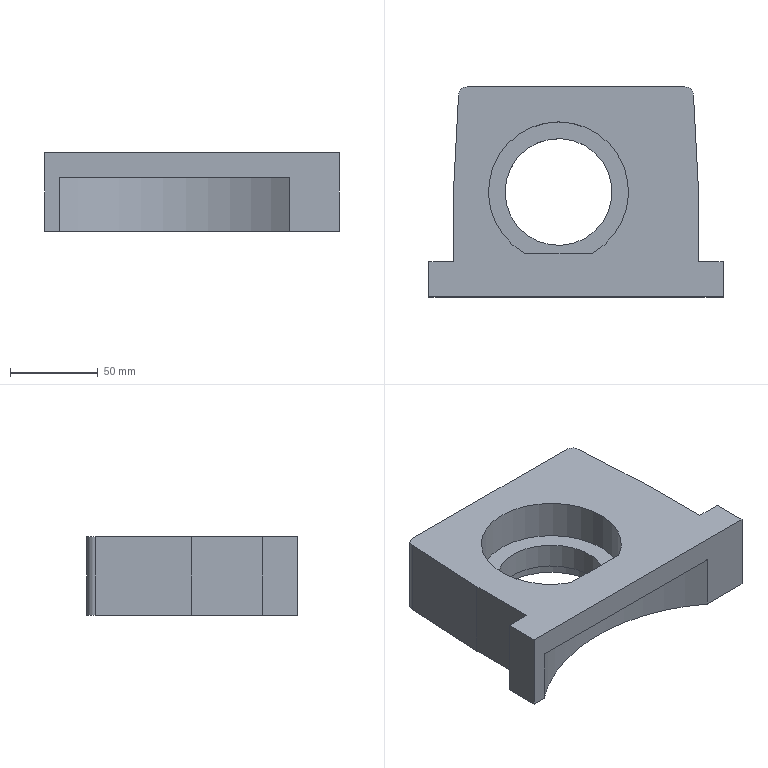Part | STEP file | SLIDE2-3_id590_x_t | 1 solid | 22 faces | box 168 x 120 x 45 mm | volume 525996 mm3 | plane 16 | cylinder 6 | commonest cylinder face diameters 10 x2 61 x1 71 x1 80 x1 217 x1
STEP:
#1=CARTESIAN_POINT('',(-60.5,0.,123.003));
#2=VERTEX_POINT('',#1);
#3=CARTESIAN_POINT('',(-30.,0.,123.003));
#4=DIRECTION('',(0.,0.,1.));
#5=DIRECTION('',(-1.,0.,0.));
#6=AXIS2_PLACEMENT_3D('',#3,#4,#5);
#7=CIRCLE('',#6,30.5);
#8=EDGE_CURVE('',#2,#2,#7,.T.);
#9=ORIENTED_EDGE('',*,*,#8,.T.);
#10=EDGE_LOOP('',(#9));
#11=FACE_BOUND('',#10,.T.);
#12=CARTESIAN_POINT('',(-65.5,0.,123.003));
#13=VERTEX_POINT('',#12);
#14=CARTESIAN_POINT('',(-30.,0.,123.003));
#15=DIRECTION('',(0.,0.,-1.));
#16=DIRECTION('',(-1.,0.,0.));
#17=AXIS2_PLACEMENT_3D('',#14,#15,#16);
#18=CIRCLE('',#17,35.5);
#19=EDGE_CURVE('',#13,#13,#18,.T.);
#20=ORIENTED_EDGE('',*,*,#19,.T.);
#21=EDGE_LOOP('',(#20));
#22=FACE_BOUND('',#21,.T.);
#23=CARTESIAN_POINT('',(50.,60.,123.003));
#24=DIRECTION('',(0.,0.,-1.));
#25=DIRECTION('',(-1.,0.,0.));
#26=AXIS2_PLACEMENT_3D('',#23,#24,#25);
#27=PLANE('',#26);
#28=ADVANCED_FACE('',(#11,#22),#27,.T.);
#29=ORIENTED_EDGE('',*,*,#19,.F.);
#30=EDGE_LOOP('',(#29));
#31=FACE_BOUND('',#30,.T.);
#32=CARTESIAN_POINT('',(-65.5,0.,115.003));
#33=VERTEX_POINT('',#32);
#34=CARTESIAN_POINT('',(-30.,0.,115.003));
#35=DIRECTION('',(0.,0.,-1.));
#36=DIRECTION('',(-1.,0.,0.));
#37=AXIS2_PLACEMENT_3D('',#34,#35,#36);
#38=CIRCLE('',#37,35.5);
#39=EDGE_CURVE('',#33,#33,#38,.T.);
#40=ORIENTED_EDGE('',*,*,#39,.T.);
#41=EDGE_LOOP('',(#40));
#42=FACE_BOUND('',#41,.T.);
#43=CARTESIAN_POINT('',(-30.,0.,115.003));
#44=DIRECTION('',(0.,0.,-1.));
#45=DIRECTION('',(-1.,0.,0.));
#46=AXIS2_PLACEMENT_3D('',#43,#44,#45);
#47=CYLINDRICAL_SURFACE('',#46,35.5);
#48=ADVANCED_FACE('',(#31,#42),#47,.F.);
#49=ORIENTED_EDGE('',*,*,#8,.F.);
#50=EDGE_LOOP('',(#49));
#51=FACE_BOUND('',#50,.T.);
#52=CARTESIAN_POINT('',(-60.5,0.,137.503));
#53=VERTEX_POINT('',#52);
#54=CARTESIAN_POINT('',(-30.,0.,137.503));
#55=DIRECTION('',(0.,0.,1.));
#56=DIRECTION('',(-1.,0.,0.));
#57=AXIS2_PLACEMENT_3D('',#54,#55,#56);
#58=CIRCLE('',#57,30.5);
#59=EDGE_CURVE('',#53,#53,#58,.T.);
#60=ORIENTED_EDGE('',*,*,#59,.T.);
#61=EDGE_LOOP('',(#60));
#62=FACE_BOUND('',#61,.T.);
#63=CARTESIAN_POINT('',(-30.,0.,123.003));
#64=DIRECTION('',(0.,0.,-1.));
#65=DIRECTION('',(-1.,0.,0.));
#66=AXIS2_PLACEMENT_3D('',#63,#64,#65);
#67=CYLINDRICAL_SURFACE('',#66,30.5);
#68=ADVANCED_FACE('',(#51,#62),#67,.F.);
#69=CARTESIAN_POINT('',(35.892,-60.,146.));
#70=VERTEX_POINT('',#69);
#71=CARTESIAN_POINT('',(-95.892,-60.,146.));
#72=VERTEX_POINT('',#71);
#73=CARTESIAN_POINT('',(-30.,-146.2,146.));
#74=DIRECTION('',(0.,0.,1.));
#75=DIRECTION('',(1.,0.,0.));
#76=AXIS2_PLACEMENT_3D('',#73,#74,#75);
#77=CIRCLE('',#76,108.5);
#78=EDGE_CURVE('',#70,#72,#77,.T.);
#79=ORIENTED_EDGE('',*,*,#78,.T.);
#80=CARTESIAN_POINT('',(-95.892,-60.,115.003));
#81=VERTEX_POINT('',#80);
#82=CARTESIAN_POINT('',(-95.892,-60.,115.003));
#83=DIRECTION('',(0.,0.,1.));
#84=VECTOR('',#83,1.);
#85=LINE('',#82,#84);
#86=EDGE_CURVE('',#81,#72,#85,.T.);
#87=ORIENTED_EDGE('',*,*,#86,.F.);
#88=CARTESIAN_POINT('',(35.892,-60.,115.003));
#89=VERTEX_POINT('',#88);
#90=CARTESIAN_POINT('',(-30.,-146.2,115.003));
#91=DIRECTION('',(0.,0.,-1.));
#92=DIRECTION('',(1.,0.,0.));
#93=AXIS2_PLACEMENT_3D('',#90,#91,#92);
#94=CIRCLE('',#93,108.5);
#95=EDGE_CURVE('',#81,#89,#94,.T.);
#96=ORIENTED_EDGE('',*,*,#95,.T.);
#97=CARTESIAN_POINT('',(35.892,-60.,115.003));
#98=DIRECTION('',(0.,0.,-1.));
#99=VECTOR('',#98,1.);
#100=LINE('',#97,#99);
#101=EDGE_CURVE('',#70,#89,#100,.T.);
#102=ORIENTED_EDGE('',*,*,#101,.F.);
#103=EDGE_LOOP('',(#79,#87,#96,#102));
#104=FACE_OUTER_BOUND('',#103,.T.);
#105=CARTESIAN_POINT('',(-30.,-146.2,146.));
#106=DIRECTION('',(0.,0.,1.));
#107=DIRECTION('',(1.,0.,0.));
#108=AXIS2_PLACEMENT_3D('',#105,#106,#107);
#109=CYLINDRICAL_SURFACE('',#108,108.5);
#110=ADVANCED_FACE('',(#104),#109,.F.);
#111=CARTESIAN_POINT('',(-98.,-60.,146.));
#112=DIRECTION('',(1.,0.,0.));
#113=VECTOR('',#112,1.);
#114=LINE('',#111,#113);
#115=EDGE_CURVE('',#72,#70,#114,.T.);
#116=ORIENTED_EDGE('',*,*,#115,.F.);
#117=ORIENTED_EDGE('',*,*,#78,.F.);
#118=EDGE_LOOP('',(#116,#117));
#119=FACE_OUTER_BOUND('',#118,.T.);
#120=CARTESIAN_POINT('',(0.,-40.,146.));
#121=DIRECTION('',(0.,0.,1.));
#122=DIRECTION('',(1.,0.,0.));
#123=AXIS2_PLACEMENT_3D('',#120,#121,#122);
#124=PLANE('',#123);
#125=ADVANCED_FACE('',(#119),#124,.F.);
#126=ORIENTED_EDGE('',*,*,#39,.F.);
#127=EDGE_LOOP('',(#126));
#128=FACE_BOUND('',#127,.T.);
#129=CARTESIAN_POINT('',(50.,-40.,115.003));
#130=VERTEX_POINT('',#129);
#131=CARTESIAN_POINT('',(50.,0.05468,115.003));
#132=VERTEX_POINT('',#131);
#133=CARTESIAN_POINT('',(50.,-50.,115.003));
#134=DIRECTION('',(0.,1.,0.));
#135=VECTOR('',#134,1.);
#136=LINE('',#133,#135);
#137=EDGE_CURVE('',#130,#132,#136,.T.);
#138=ORIENTED_EDGE('',*,*,#137,.F.);
#139=CARTESIAN_POINT('',(64.,-40.,115.003));
#140=VERTEX_POINT('',#139);
#141=CARTESIAN_POINT('',(58.,-40.,115.003));
#142=DIRECTION('',(-1.,0.,0.));
#143=VECTOR('',#142,1.);
#144=LINE('',#141,#143);
#145=EDGE_CURVE('',#140,#130,#144,.T.);
#146=ORIENTED_EDGE('',*,*,#145,.F.);
#147=CARTESIAN_POINT('',(64.,-60.,115.003));
#148=VERTEX_POINT('',#147);
#149=CARTESIAN_POINT('',(64.,-60.,115.003));
#150=DIRECTION('',(0.,1.,0.));
#151=VECTOR('',#150,1.);
#152=LINE('',#149,#151);
#153=EDGE_CURVE('',#148,#140,#152,.T.);
#154=ORIENTED_EDGE('',*,*,#153,.F.);
#155=CARTESIAN_POINT('',(-98.,-60.,115.003));
#156=DIRECTION('',(1.,0.,0.));
#157=VECTOR('',#156,1.);
#158=LINE('',#155,#157);
#159=EDGE_CURVE('',#89,#148,#158,.T.);
#160=ORIENTED_EDGE('',*,*,#159,.F.);
#161=ORIENTED_EDGE('',*,*,#95,.F.);
#162=CARTESIAN_POINT('',(-104.,-60.,115.003));
#163=VERTEX_POINT('',#162);
#164=CARTESIAN_POINT('',(-98.,-60.,115.003));
#165=DIRECTION('',(1.,0.,0.));
#166=VECTOR('',#165,1.);
#167=LINE('',#164,#166);
#168=EDGE_CURVE('',#163,#81,#167,.T.);
#169=ORIENTED_EDGE('',*,*,#168,.F.);
#170=CARTESIAN_POINT('',(-104.,-40.,115.003));
#171=VERTEX_POINT('',#170);
#172=CARTESIAN_POINT('',(-104.,-50.,115.003));
#173=DIRECTION('',(0.,-1.,0.));
#174=VECTOR('',#173,1.);
#175=LINE('',#172,#174);
#176=EDGE_CURVE('',#171,#163,#175,.T.);
#177=ORIENTED_EDGE('',*,*,#176,.F.);
#178=CARTESIAN_POINT('',(-90.,-40.,115.003));
#179=VERTEX_POINT('',#178);
#180=CARTESIAN_POINT('',(-90.,-40.,115.003));
#181=DIRECTION('',(-1.,0.,0.));
#182=VECTOR('',#181,1.);
#183=LINE('',#180,#182);
#184=EDGE_CURVE('',#179,#171,#183,.T.);
#185=ORIENTED_EDGE('',*,*,#184,.F.);
#186=CARTESIAN_POINT('',(-90.,0.05468,115.003));
#187=VERTEX_POINT('',#186);
#188=CARTESIAN_POINT('',(-90.,60.,115.003));
#189=DIRECTION('',(0.,-1.,0.));
#190=VECTOR('',#189,1.);
#191=LINE('',#188,#190);
#192=EDGE_CURVE('',#187,#179,#191,.T.);
#193=ORIENTED_EDGE('',*,*,#192,.F.);
#194=CARTESIAN_POINT('',(-87.107,55.262,115.003));
#195=VERTEX_POINT('',#194);
#196=CARTESIAN_POINT('',(-87.107,55.262,115.003));
#197=DIRECTION('',(0.05234,0.9986,0.));
#198=VECTOR('',#197,1.);
#199=LINE('',#196,#198);
#200=EDGE_CURVE('',#187,#195,#199,.T.);
#201=ORIENTED_EDGE('',*,*,#200,.T.);
#202=CARTESIAN_POINT('',(-82.114,60.,115.003));
#203=VERTEX_POINT('',#202);
#204=CARTESIAN_POINT('',(-82.114,55.,115.003));
#205=DIRECTION('',(0.,0.,1.));
#206=DIRECTION('',(-1.,0.,0.));
#207=AXIS2_PLACEMENT_3D('',#204,#205,#206);
#208=CIRCLE('',#207,5.);
#209=EDGE_CURVE('',#203,#195,#208,.T.);
#210=ORIENTED_EDGE('',*,*,#209,.F.);
#211=CARTESIAN_POINT('',(42.114,60.,115.003));
#212=VERTEX_POINT('',#211);
#213=CARTESIAN_POINT('',(50.,60.,115.003));
#214=DIRECTION('',(-1.,0.,0.));
#215=VECTOR('',#214,1.);
#216=LINE('',#213,#215);
#217=EDGE_CURVE('',#212,#203,#216,.T.);
#218=ORIENTED_EDGE('',*,*,#217,.F.);
#219=CARTESIAN_POINT('',(47.107,55.262,115.003));
#220=VERTEX_POINT('',#219);
#221=CARTESIAN_POINT('',(42.114,55.,115.003));
#222=DIRECTION('',(0.,0.,1.));
#223=DIRECTION('',(-1.,0.,0.));
#224=AXIS2_PLACEMENT_3D('',#221,#222,#223);
#225=CIRCLE('',#224,5.);
#226=EDGE_CURVE('',#220,#212,#225,.T.);
#227=ORIENTED_EDGE('',*,*,#226,.F.);
#228=CARTESIAN_POINT('',(50.,0.05468,115.003));
#229=DIRECTION('',(0.05234,-0.9986,0.));
#230=VECTOR('',#229,1.);
#231=LINE('',#228,#230);
#232=EDGE_CURVE('',#220,#132,#231,.T.);
#233=ORIENTED_EDGE('',*,*,#232,.T.);
#234=EDGE_LOOP('',(#138,#146,#154,#160,#161,#169,#177,#185,#193,#201,#210,#218,#227,#233));
#235=FACE_BOUND('',#234,.T.);
#236=CARTESIAN_POINT('',(50.5,0.,115.003));
#237=DIRECTION('',(0.,0.,1.));
#238=DIRECTION('',(1.,0.,0.));
#239=AXIS2_PLACEMENT_3D('',#236,#237,#238);
#240=PLANE('',#239);
#241=ADVANCED_FACE('',(#128,#235),#240,.F.);
#242=ORIENTED_EDGE('',*,*,#59,.F.);
#243=EDGE_LOOP('',(#242));
#244=FACE_BOUND('',#243,.T.);
#245=CARTESIAN_POINT('',(-10.635,-35.,137.503));
#246=VERTEX_POINT('',#245);
#247=CARTESIAN_POINT('',(-49.365,-35.,137.503));
#248=VERTEX_POINT('',#247);
#249=CARTESIAN_POINT('',(-30.,0.,137.503));
#250=DIRECTION('',(0.,0.,1.));
#251=DIRECTION('',(-1.,0.,0.));
#252=AXIS2_PLACEMENT_3D('',#249,#250,#251);
#253=CIRCLE('',#252,40.);
#254=EDGE_CURVE('',#246,#248,#253,.T.);
#255=ORIENTED_EDGE('',*,*,#254,.T.);
#256=CARTESIAN_POINT('',(-10.635,-35.,137.503));
#257=DIRECTION('',(-1.,0.,0.));
#258=VECTOR('',#257,1.);
#259=LINE('',#256,#258);
#260=EDGE_CURVE('',#246,#248,#259,.T.);
#261=ORIENTED_EDGE('',*,*,#260,.F.);
#262=EDGE_LOOP('',(#255,#261));
#263=FACE_BOUND('',#262,.T.);
#264=CARTESIAN_POINT('',(50.,60.,137.503));
#265=DIRECTION('',(0.,0.,-1.));
#266=DIRECTION('',(-1.,0.,0.));
#267=AXIS2_PLACEMENT_3D('',#264,#265,#266);
#268=PLANE('',#267);
#269=ADVANCED_FACE('',(#244,#263),#268,.F.);
#270=CARTESIAN_POINT('',(42.114,60.,160.003));
#271=VERTEX_POINT('',#270);
#272=CARTESIAN_POINT('',(-82.114,60.,160.003));
#273=VERTEX_POINT('',#272);
#274=CARTESIAN_POINT('',(50.5,60.,160.003));
#275=DIRECTION('',(-1.,0.,0.));
#276=VECTOR('',#275,1.);
#277=LINE('',#274,#276);
#278=EDGE_CURVE('',#271,#273,#277,.T.);
#279=ORIENTED_EDGE('',*,*,#278,.F.);
#280=CARTESIAN_POINT('',(42.114,60.,115.003));
#281=DIRECTION('',(0.,0.,1.));
#282=VECTOR('',#281,1.);
#283=LINE('',#280,#282);
#284=EDGE_CURVE('',#212,#271,#283,.T.);
#285=ORIENTED_EDGE('',*,*,#284,.F.);
#286=ORIENTED_EDGE('',*,*,#217,.T.);
#287=CARTESIAN_POINT('',(-82.114,60.,115.003));
#288=DIRECTION('',(0.,0.,-1.));
#289=VECTOR('',#288,1.);
#290=LINE('',#287,#289);
#291=EDGE_CURVE('',#273,#203,#290,.T.);
#292=ORIENTED_EDGE('',*,*,#291,.F.);
#293=EDGE_LOOP('',(#279,#285,#286,#292));
#294=FACE_OUTER_BOUND('',#293,.T.);
#295=CARTESIAN_POINT('',(50.,60.,115.003));
#296=DIRECTION('',(0.,1.,0.));
#297=DIRECTION('',(0.,0.,1.));
#298=AXIS2_PLACEMENT_3D('',#295,#296,#297);
#299=PLANE('',#298);
#300=ADVANCED_FACE('',(#294),#299,.T.);
#301=ORIENTED_EDGE('',*,*,#291,.T.);
#302=ORIENTED_EDGE('',*,*,#209,.T.);
#303=CARTESIAN_POINT('',(-87.107,55.262,160.003));
#304=VERTEX_POINT('',#303);
#305=CARTESIAN_POINT('',(-87.107,55.262,115.003));
#306=DIRECTION('',(0.,0.,1.));
#307=VECTOR('',#306,1.);
#308=LINE('',#305,#307);
#309=EDGE_CURVE('',#195,#304,#308,.T.);
#310=ORIENTED_EDGE('',*,*,#309,.T.);
#311=CARTESIAN_POINT('',(-82.114,55.,160.003));
#312=DIRECTION('',(0.,0.,1.));
#313=DIRECTION('',(-1.,0.,0.));
#314=AXIS2_PLACEMENT_3D('',#311,#312,#313);
#315=CIRCLE('',#314,5.);
#316=EDGE_CURVE('',#273,#304,#315,.T.);
#317=ORIENTED_EDGE('',*,*,#316,.F.);
#318=EDGE_LOOP('',(#301,#302,#310,#317));
#319=FACE_OUTER_BOUND('',#318,.T.);
#320=CARTESIAN_POINT('',(-82.114,55.,115.003));
#321=DIRECTION('',(0.,0.,-1.));
#322=DIRECTION('',(-1.,0.,0.));
#323=AXIS2_PLACEMENT_3D('',#320,#321,#322);
#324=CYLINDRICAL_SURFACE('',#323,5.);
#325=ADVANCED_FACE('',(#319),#324,.T.);
#326=CARTESIAN_POINT('',(-90.,0.05468,160.003));
#327=VERTEX_POINT('',#326);
#328=CARTESIAN_POINT('',(-87.107,55.262,160.003));
#329=DIRECTION('',(-0.05234,-0.9986,0.));
#330=VECTOR('',#329,1.);
#331=LINE('',#328,#330);
#332=EDGE_CURVE('',#304,#327,#331,.T.);
#333=ORIENTED_EDGE('',*,*,#332,.F.);
#334=ORIENTED_EDGE('',*,*,#309,.F.);
#335=ORIENTED_EDGE('',*,*,#200,.F.);
#336=CARTESIAN_POINT('',(-90.,0.05468,115.003));
#337=DIRECTION('',(0.,0.,-1.));
#338=VECTOR('',#337,1.);
#339=LINE('',#336,#338);
#340=EDGE_CURVE('',#327,#187,#339,.T.);
#341=ORIENTED_EDGE('',*,*,#340,.F.);
#342=EDGE_LOOP('',(#333,#334,#335,#341));
#343=FACE_OUTER_BOUND('',#342,.T.);
#344=CARTESIAN_POINT('',(-87.107,55.262,115.003));
#345=DIRECTION('',(0.9986,-0.05234,0.));
#346=DIRECTION('',(0.05234,0.9986,0.));
#347=AXIS2_PLACEMENT_3D('',#344,#345,#346);
#348=PLANE('',#347);
#349=ADVANCED_FACE('',(#343),#348,.F.);
#350=CARTESIAN_POINT('',(-90.,-40.,160.003));
#351=VERTEX_POINT('',#350);
#352=CARTESIAN_POINT('',(-90.,0.,160.003));
#353=DIRECTION('',(0.,-1.,0.));
#354=VECTOR('',#353,1.);
#355=LINE('',#352,#354);
#356=EDGE_CURVE('',#327,#351,#355,.T.);
#357=ORIENTED_EDGE('',*,*,#356,.F.);
#358=ORIENTED_EDGE('',*,*,#340,.T.);
#359=ORIENTED_EDGE('',*,*,#192,.T.);
#360=CARTESIAN_POINT('',(-90.,-40.,115.003));
#361=DIRECTION('',(0.,0.,-1.));
#362=VECTOR('',#361,1.);
#363=LINE('',#360,#362);
#364=EDGE_CURVE('',#351,#179,#363,.T.);
#365=ORIENTED_EDGE('',*,*,#364,.F.);
#366=EDGE_LOOP('',(#357,#358,#359,#365));
#367=FACE_OUTER_BOUND('',#366,.T.);
#368=CARTESIAN_POINT('',(-90.,60.,115.003));
#369=DIRECTION('',(-1.,0.,0.));
#370=DIRECTION('',(0.,0.,1.));
#371=AXIS2_PLACEMENT_3D('',#368,#369,#370);
#372=PLANE('',#371);
#373=ADVANCED_FACE('',(#367),#372,.T.);
#374=ORIENTED_EDGE('',*,*,#364,.T.);
#375=ORIENTED_EDGE('',*,*,#184,.T.);
#376=CARTESIAN_POINT('',(-104.,-40.,160.003));
#377=VERTEX_POINT('',#376);
#378=CARTESIAN_POINT('',(-104.,-40.,115.003));
#379=DIRECTION('',(0.,0.,-1.));
#380=VECTOR('',#379,1.);
#381=LINE('',#378,#380);
#382=EDGE_CURVE('',#377,#171,#381,.T.);
#383=ORIENTED_EDGE('',*,*,#382,.F.);
#384=CARTESIAN_POINT('',(50.5,-40.,160.003));
#385=DIRECTION('',(-1.,0.,0.));
#386=VECTOR('',#385,1.);
#387=LINE('',#384,#386);
#388=EDGE_CURVE('',#351,#377,#387,.T.);
#389=ORIENTED_EDGE('',*,*,#388,.F.);
#390=EDGE_LOOP('',(#374,#375,#383,#389));
#391=FACE_OUTER_BOUND('',#390,.T.);
#392=CARTESIAN_POINT('',(-90.,-40.,115.003));
#393=DIRECTION('',(0.,1.,0.));
#394=DIRECTION('',(0.,0.,1.));
#395=AXIS2_PLACEMENT_3D('',#392,#393,#394);
#396=PLANE('',#395);
#397=ADVANCED_FACE('',(#391),#396,.T.);
#398=ORIENTED_EDGE('',*,*,#382,.T.);
#399=ORIENTED_EDGE('',*,*,#176,.T.);
#400=CARTESIAN_POINT('',(-104.,-60.,160.003));
#401=VERTEX_POINT('',#400);
#402=CARTESIAN_POINT('',(-104.,-60.,115.003));
#403=DIRECTION('',(0.,0.,-1.));
#404=VECTOR('',#403,1.);
#405=LINE('',#402,#404);
#406=EDGE_CURVE('',#401,#163,#405,.T.);
#407=ORIENTED_EDGE('',*,*,#406,.F.);
#408=CARTESIAN_POINT('',(-104.,0.,160.003));
#409=DIRECTION('',(0.,-1.,0.));
#410=VECTOR('',#409,1.);
#411=LINE('',#408,#410);
#412=EDGE_CURVE('',#377,#401,#411,.T.);
#413=ORIENTED_EDGE('',*,*,#412,.F.);
#414=EDGE_LOOP('',(#398,#399,#407,#413));
#415=FACE_OUTER_BOUND('',#414,.T.);
#416=CARTESIAN_POINT('',(-104.,-50.,115.003));
#417=DIRECTION('',(-1.,0.,0.));
#418=DIRECTION('',(0.,0.,1.));
#419=AXIS2_PLACEMENT_3D('',#416,#417,#418);
#420=PLANE('',#419);
#421=ADVANCED_FACE('',(#415),#420,.T.);
#422=ORIENTED_EDGE('',*,*,#86,.T.);
#423=ORIENTED_EDGE('',*,*,#115,.T.);
#424=ORIENTED_EDGE('',*,*,#101,.T.);
#425=ORIENTED_EDGE('',*,*,#159,.T.);
#426=CARTESIAN_POINT('',(64.,-60.,160.003));
#427=VERTEX_POINT('',#426);
#428=CARTESIAN_POINT('',(64.,-60.,115.003));
#429=DIRECTION('',(0.,0.,-1.));
#430=VECTOR('',#429,1.);
#431=LINE('',#428,#430);
#432=EDGE_CURVE('',#427,#148,#431,.T.);
#433=ORIENTED_EDGE('',*,*,#432,.F.);
#434=CARTESIAN_POINT('',(50.5,-60.,160.003));
#435=DIRECTION('',(1.,0.,0.));
#436=VECTOR('',#435,1.);
#437=LINE('',#434,#436);
#438=EDGE_CURVE('',#401,#427,#437,.T.);
#439=ORIENTED_EDGE('',*,*,#438,.F.);
#440=ORIENTED_EDGE('',*,*,#406,.T.);
#441=ORIENTED_EDGE('',*,*,#168,.T.);
#442=EDGE_LOOP('',(#422,#423,#424,#425,#433,#439,#440,#441));
#443=FACE_OUTER_BOUND('',#442,.T.);
#444=CARTESIAN_POINT('',(-98.,-60.,115.003));
#445=DIRECTION('',(0.,-1.,0.));
#446=DIRECTION('',(0.,0.,-1.));
#447=AXIS2_PLACEMENT_3D('',#444,#445,#446);
#448=PLANE('',#447);
#449=ADVANCED_FACE('',(#443),#448,.T.);
#450=ORIENTED_EDGE('',*,*,#432,.T.);
#451=ORIENTED_EDGE('',*,*,#153,.T.);
#452=CARTESIAN_POINT('',(64.,-40.,160.003));
#453=VERTEX_POINT('',#452);
#454=CARTESIAN_POINT('',(64.,-40.,115.003));
#455=DIRECTION('',(0.,0.,-1.));
#456=VECTOR('',#455,1.);
#457=LINE('',#454,#456);
#458=EDGE_CURVE('',#453,#140,#457,.T.);
#459=ORIENTED_EDGE('',*,*,#458,.F.);
#460=CARTESIAN_POINT('',(64.,0.,160.003));
#461=DIRECTION('',(0.,1.,0.));
#462=VECTOR('',#461,1.);
#463=LINE('',#460,#462);
#464=EDGE_CURVE('',#427,#453,#463,.T.);
#465=ORIENTED_EDGE('',*,*,#464,.F.);
#466=EDGE_LOOP('',(#450,#451,#459,#465));
#467=FACE_OUTER_BOUND('',#466,.T.);
#468=CARTESIAN_POINT('',(64.,-60.,115.003));
#469=DIRECTION('',(1.,0.,0.));
#470=DIRECTION('',(0.,0.,-1.));
#471=AXIS2_PLACEMENT_3D('',#468,#469,#470);
#472=PLANE('',#471);
#473=ADVANCED_FACE('',(#467),#472,.T.);
#474=ORIENTED_EDGE('',*,*,#458,.T.);
#475=ORIENTED_EDGE('',*,*,#145,.T.);
#476=CARTESIAN_POINT('',(50.,-40.,160.003));
#477=VERTEX_POINT('',#476);
#478=CARTESIAN_POINT('',(50.,-40.,115.003));
#479=DIRECTION('',(0.,0.,-1.));
#480=VECTOR('',#479,1.);
#481=LINE('',#478,#480);
#482=EDGE_CURVE('',#477,#130,#481,.T.);
#483=ORIENTED_EDGE('',*,*,#482,.F.);
#484=CARTESIAN_POINT('',(50.5,-40.,160.003));
#485=DIRECTION('',(-1.,0.,0.));
#486=VECTOR('',#485,1.);
#487=LINE('',#484,#486);
#488=EDGE_CURVE('',#453,#477,#487,.T.);
#489=ORIENTED_EDGE('',*,*,#488,.F.);
#490=EDGE_LOOP('',(#474,#475,#483,#489));
#491=FACE_OUTER_BOUND('',#490,.T.);
#492=CARTESIAN_POINT('',(58.,-40.,115.003));
#493=DIRECTION('',(0.,1.,0.));
#494=DIRECTION('',(0.,0.,1.));
#495=AXIS2_PLACEMENT_3D('',#492,#493,#494);
#496=PLANE('',#495);
#497=ADVANCED_FACE('',(#491),#496,.T.);
#498=ORIENTED_EDGE('',*,*,#137,.T.);
#499=CARTESIAN_POINT('',(50.,0.05468,160.003));
#500=VERTEX_POINT('',#499);
#501=CARTESIAN_POINT('',(50.,0.05468,115.003));
#502=DIRECTION('',(0.,0.,1.));
#503=VECTOR('',#502,1.);
#504=LINE('',#501,#503);
#505=EDGE_CURVE('',#132,#500,#504,.T.);
#506=ORIENTED_EDGE('',*,*,#505,.T.);
#507=CARTESIAN_POINT('',(50.,0.,160.003));
#508=DIRECTION('',(0.,1.,0.));
#509=VECTOR('',#508,1.);
#510=LINE('',#507,#509);
#511=EDGE_CURVE('',#477,#500,#510,.T.);
#512=ORIENTED_EDGE('',*,*,#511,.F.);
#513=ORIENTED_EDGE('',*,*,#482,.T.);
#514=EDGE_LOOP('',(#498,#506,#512,#513));
#515=FACE_OUTER_BOUND('',#514,.T.);
#516=CARTESIAN_POINT('',(50.,-50.,115.003));
#517=DIRECTION('',(1.,0.,0.));
#518=DIRECTION('',(0.,0.,-1.));
#519=AXIS2_PLACEMENT_3D('',#516,#517,#518);
#520=PLANE('',#519);
#521=ADVANCED_FACE('',(#515),#520,.T.);
#522=CARTESIAN_POINT('',(47.107,55.262,160.003));
#523=VERTEX_POINT('',#522);
#524=CARTESIAN_POINT('',(50.,0.05468,160.003));
#525=DIRECTION('',(-0.05234,0.9986,0.));
#526=VECTOR('',#525,1.);
#527=LINE('',#524,#526);
#528=EDGE_CURVE('',#500,#523,#527,.T.);
#529=ORIENTED_EDGE('',*,*,#528,.F.);
#530=ORIENTED_EDGE('',*,*,#505,.F.);
#531=ORIENTED_EDGE('',*,*,#232,.F.);
#532=CARTESIAN_POINT('',(47.107,55.262,115.003));
#533=DIRECTION('',(0.,0.,-1.));
#534=VECTOR('',#533,1.);
#535=LINE('',#532,#534);
#536=EDGE_CURVE('',#523,#220,#535,.T.);
#537=ORIENTED_EDGE('',*,*,#536,.F.);
#538=EDGE_LOOP('',(#529,#530,#531,#537));
#539=FACE_OUTER_BOUND('',#538,.T.);
#540=CARTESIAN_POINT('',(50.,0.05468,115.003));
#541=DIRECTION('',(-0.9986,-0.05234,0.));
#542=DIRECTION('',(0.05234,-0.9986,0.));
#543=AXIS2_PLACEMENT_3D('',#540,#541,#542);
#544=PLANE('',#543);
#545=ADVANCED_FACE('',(#539),#544,.F.);
#546=ORIENTED_EDGE('',*,*,#536,.T.);
#547=ORIENTED_EDGE('',*,*,#226,.T.);
#548=ORIENTED_EDGE('',*,*,#284,.T.);
#549=CARTESIAN_POINT('',(42.114,55.,160.003));
#550=DIRECTION('',(0.,0.,1.));
#551=DIRECTION('',(-1.,0.,0.));
#552=AXIS2_PLACEMENT_3D('',#549,#550,#551);
#553=CIRCLE('',#552,5.);
#554=EDGE_CURVE('',#523,#271,#553,.T.);
#555=ORIENTED_EDGE('',*,*,#554,.F.);
#556=EDGE_LOOP('',(#546,#547,#548,#555));
#557=FACE_OUTER_BOUND('',#556,.T.);
#558=CARTESIAN_POINT('',(42.114,55.,115.003));
#559=DIRECTION('',(0.,0.,-1.));
#560=DIRECTION('',(-1.,0.,0.));
#561=AXIS2_PLACEMENT_3D('',#558,#559,#560);
#562=CYLINDRICAL_SURFACE('',#561,5.);
#563=ADVANCED_FACE('',(#557),#562,.T.);
#564=CARTESIAN_POINT('',(-10.635,-35.,160.003));
#565=VERTEX_POINT('',#564);
#566=CARTESIAN_POINT('',(-10.635,-35.,137.503));
#567=DIRECTION('',(0.,0.,-1.));
#568=VECTOR('',#567,1.);
#569=LINE('',#566,#568);
#570=EDGE_CURVE('',#565,#246,#569,.T.);
#571=ORIENTED_EDGE('',*,*,#570,.T.);
#572=ORIENTED_EDGE('',*,*,#260,.T.);
#573=CARTESIAN_POINT('',(-49.365,-35.,160.003));
#574=VERTEX_POINT('',#573);
#575=CARTESIAN_POINT('',(-49.365,-35.,137.503));
#576=DIRECTION('',(0.,0.,1.));
#577=VECTOR('',#576,1.);
#578=LINE('',#575,#577);
#579=EDGE_CURVE('',#248,#574,#578,.T.);
#580=ORIENTED_EDGE('',*,*,#579,.T.);
#581=CARTESIAN_POINT('',(50.5,-35.,160.003));
#582=DIRECTION('',(-1.,0.,0.));
#583=VECTOR('',#582,1.);
#584=LINE('',#581,#583);
#585=EDGE_CURVE('',#565,#574,#584,.T.);
#586=ORIENTED_EDGE('',*,*,#585,.F.);
#587=EDGE_LOOP('',(#571,#572,#580,#586));
#588=FACE_OUTER_BOUND('',#587,.T.);
#589=CARTESIAN_POINT('',(-10.635,-35.,137.503));
#590=DIRECTION('',(0.,1.,0.));
#591=DIRECTION('',(0.,0.,1.));
#592=AXIS2_PLACEMENT_3D('',#589,#590,#591);
#593=PLANE('',#592);
#594=ADVANCED_FACE('',(#588),#593,.T.);
#595=CARTESIAN_POINT('',(-30.,0.,160.003));
#596=DIRECTION('',(0.,0.,-1.));
#597=DIRECTION('',(-1.,0.,0.));
#598=AXIS2_PLACEMENT_3D('',#595,#596,#597);
#599=CIRCLE('',#598,40.);
#600=EDGE_CURVE('',#574,#565,#599,.T.);
#601=ORIENTED_EDGE('',*,*,#600,.F.);
#602=ORIENTED_EDGE('',*,*,#579,.F.);
#603=ORIENTED_EDGE('',*,*,#254,.F.);
#604=ORIENTED_EDGE('',*,*,#570,.F.);
#605=EDGE_LOOP('',(#601,#602,#603,#604));
#606=FACE_OUTER_BOUND('',#605,.T.);
#607=CARTESIAN_POINT('',(-30.,0.,137.503));
#608=DIRECTION('',(0.,0.,-1.));
#609=DIRECTION('',(-1.,0.,0.));
#610=AXIS2_PLACEMENT_3D('',#607,#608,#609);
#611=CYLINDRICAL_SURFACE('',#610,40.);
#612=ADVANCED_FACE('',(#606),#611,.F.);
#613=ORIENTED_EDGE('',*,*,#585,.T.);
#614=ORIENTED_EDGE('',*,*,#600,.T.);
#615=EDGE_LOOP('',(#613,#614));
#616=FACE_BOUND('',#615,.T.);
#617=ORIENTED_EDGE('',*,*,#528,.T.);
#618=ORIENTED_EDGE('',*,*,#554,.T.);
#619=ORIENTED_EDGE('',*,*,#278,.T.);
#620=ORIENTED_EDGE('',*,*,#316,.T.);
#621=ORIENTED_EDGE('',*,*,#332,.T.);
#622=ORIENTED_EDGE('',*,*,#356,.T.);
#623=ORIENTED_EDGE('',*,*,#388,.T.);
#624=ORIENTED_EDGE('',*,*,#412,.T.);
#625=ORIENTED_EDGE('',*,*,#438,.T.);
#626=ORIENTED_EDGE('',*,*,#464,.T.);
#627=ORIENTED_EDGE('',*,*,#488,.T.);
#628=ORIENTED_EDGE('',*,*,#511,.T.);
#629=EDGE_LOOP('',(#617,#618,#619,#620,#621,#622,#623,#624,#625,#626,#627,#628));
#630=FACE_BOUND('',#629,.T.);
#631=CARTESIAN_POINT('',(50.5,0.,160.003));
#632=DIRECTION('',(0.,0.,1.));
#633=DIRECTION('',(1.,0.,0.));
#634=AXIS2_PLACEMENT_3D('',#631,#632,#633);
#635=PLANE('',#634);
#636=ADVANCED_FACE('',(#616,#630),#635,.T.);
#637=CLOSED_SHELL('',(#28,#48,#68,#110,#125,#241,#269,#300,#325,#349,#373,#397,#421,#449,#473,#497,#521,#545,#563,#594,#612,#636));
#638=MANIFOLD_SOLID_BREP('',#637);
#639=(LENGTH_UNIT()NAMED_UNIT(*)SI_UNIT(.MILLI.,.METRE.));
#640=UNCERTAINTY_MEASURE_WITH_UNIT(LENGTH_MEASURE(0.00004123),#639,'','');
#641=(NAMED_UNIT(*)PLANE_ANGLE_UNIT()SI_UNIT($,.RADIAN.));
#642=PLANE_ANGLE_MEASURE_WITH_UNIT(PLANE_ANGLE_MEASURE(0.01745),#641);
#643=DIMENSIONAL_EXPONENTS(0.,0.,0.,0.,0.,0.,0.);
#644=(CONVERSION_BASED_UNIT('DEGREE',#642)NAMED_UNIT(#643)PLANE_ANGLE_UNIT());
#645=(NAMED_UNIT(*)SI_UNIT($,.STERADIAN.)SOLID_ANGLE_UNIT());
#646=(GEOMETRIC_REPRESENTATION_CONTEXT(3)GLOBAL_UNCERTAINTY_ASSIGNED_CONTEXT((#640))GLOBAL_UNIT_ASSIGNED_CONTEXT((#639,#644,#645))REPRESENTATION_CONTEXT('',''));
#647=ADVANCED_BREP_SHAPE_REPRESENTATION('',(#638),#646);